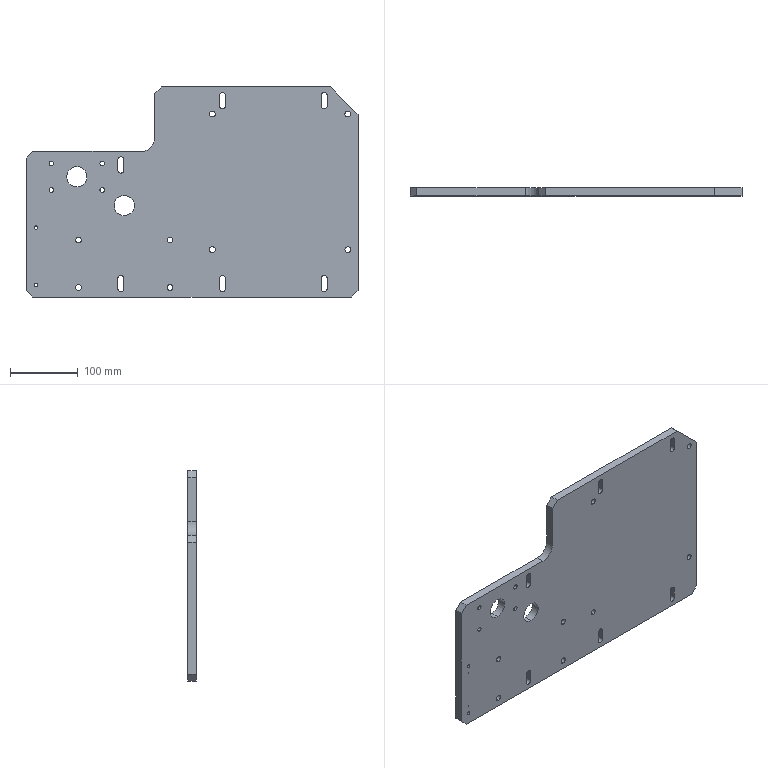Part | STEP file | PN_0035 | 1 solid | 92 faces | box 490 x 12 x 310 mm | volume 1555006 mm3 | cylinder 59 | plane 25 | cone 8 | commonest cylinder face diameters 9 x18 8.5 x16 5 x8 6.8 x8 8 x4 30 x4